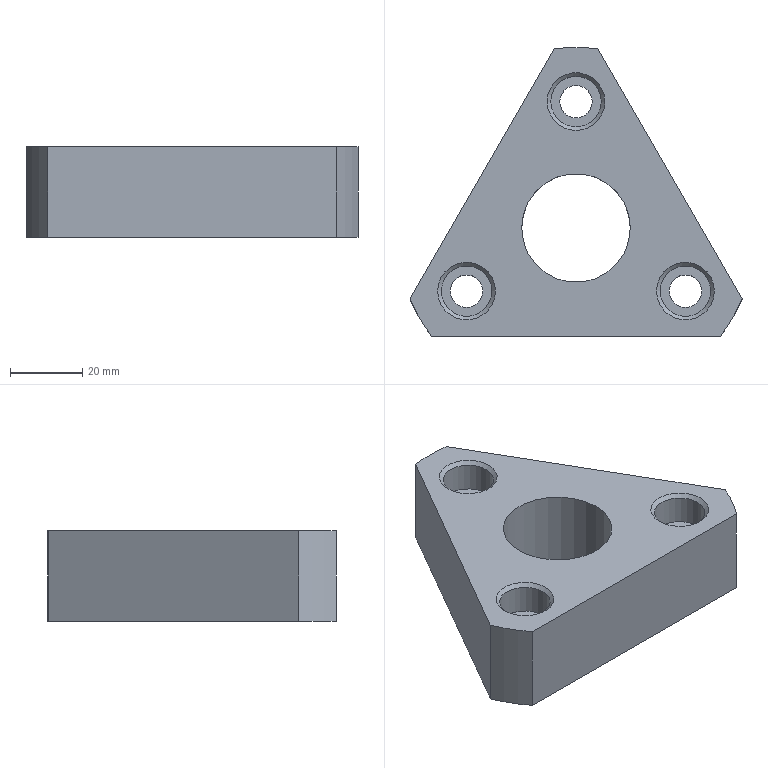NC program | NX | posted with a generic post | part box 91.962 x 80 x 25 mm
Lines 5877 to 6623 of 11626:
(ZLEVEL_PROFILE , TOOL : D10)
N11722 T10 M6
N11724 G54
N11726 G17 G0 G90 X-28.502 Y-26.671 S3000 M3
N11728 G43 Z30. H10
N11730 Z2.
N11732 G94 G1 X-28.584 Y-26.447 Z1.994 F1000.
N11734 X-29.091 Y-25.883 Z1.974
N11736 X-29.773 Y-25.55 Z1.954
N11738 X-30.128 Y-25.517 Z1.945
N11740 X-30.436 Y-25.474 Z1.937
N11742 X-30.736 Y-25.519 Z1.929
N11744 X-31.068 Y-25.672 Z1.919
N11746 X-31.388 Y-25.8 Z1.91
N11748 X-31.928 Y-26.291 Z1.891
N11750 X-32.255 Y-26.944 Z1.872
N11752 X-32.292 Y-27.286 Z1.863
N11754 X-32.325 Y-27.518 Z1.857
N11756 X-32.211 Y-28.178 Z1.839
N11758 X-31.886 Y-28.758 Z1.822
N11760 X-31.388 Y-29.199 Z1.804
N11762 X-31.068 Y-29.328 Z1.795
N11764 X-30.595 Y-29.446 Z1.782
N11766 X-30.449 Y-29.483 Z1.779
N11768 X-30.113 Y-29.481 Z1.77
N11770 X-29.771 Y-29.451 Z1.761
N11772 X-29.121 Y-29.141 Z1.742
N11774 X-28.626 Y-28.618 Z1.723
N11776 X-28.472 Y-28.252 Z1.713
N11778 X-28.337 Y-27.96 Z1.704
N11780 X-28.329 Y-27.504 Z1.692
N11782 X-28.324 Y-27.16 Z1.683
N11784 X-28.584 Y-26.447 Z1.663
N11786 X-29.091 Y-25.883 Z1.643
N11788 X-29.773 Y-25.55 Z1.624
N11790 X-30.128 Y-25.517 Z1.614
N11792 X-30.436 Y-25.474 Z1.606
N11794 X-30.736 Y-25.519 Z1.598
N11796 X-31.068 Y-25.672 Z1.589
N11798 X-31.388 Y-25.8 Z1.58
N11800 X-31.928 Y-26.291 Z1.56
N11802 X-32.255 Y-26.944 Z1.541
N11804 X-32.292 Y-27.286 Z1.532
N11806 X-32.325 Y-27.518 Z1.526
N11808 X-32.211 Y-28.178 Z1.509
N11810 X-31.886 Y-28.758 Z1.491
N11812 X-31.388 Y-29.199 Z1.474
N11814 X-31.068 Y-29.328 Z1.465
N11816 X-30.595 Y-29.446 Z1.452
N11818 X-30.449 Y-29.483 Z1.448
N11820 X-30.113 Y-29.481 Z1.439
N11822 X-29.771 Y-29.451 Z1.43
N11824 X-29.121 Y-29.141 Z1.411
N11826 X-28.626 Y-28.618 Z1.393
N11828 X-28.472 Y-28.252 Z1.382
N11830 X-28.337 Y-27.96 Z1.374
N11832 X-28.329 Y-27.504 Z1.362
N11834 X-28.324 Y-27.16 Z1.353
N11836 X-28.584 Y-26.447 Z1.333
N11838 X-29.091 Y-25.883 Z1.313
N11840 X-29.773 Y-25.55 Z1.293
N11842 X-30.128 Y-25.517 Z1.284
N11844 X-30.436 Y-25.474 Z1.276
N11846 X-30.736 Y-25.519 Z1.268
N11848 X-31.068 Y-25.672 Z1.258
N11850 X-31.388 Y-25.8 Z1.249
N11852 X-31.928 Y-26.291 Z1.23
N11854 X-32.255 Y-26.944 Z1.211
N11856 X-32.292 Y-27.286 Z1.202
N11858 X-32.325 Y-27.518 Z1.196
N11860 X-32.211 Y-28.178 Z1.178
N11862 X-31.886 Y-28.758 Z1.161
N11864 X-31.388 Y-29.199 Z1.143
N11866 X-31.068 Y-29.328 Z1.134
N11868 X-30.595 Y-29.446 Z1.122
N11870 X-30.449 Y-29.483 Z1.118
N11872 X-30.113 Y-29.481 Z1.109
N11874 X-29.771 Y-29.451 Z1.1
N11876 X-29.121 Y-29.141 Z1.081
N11878 X-28.626 Y-28.618 Z1.062
N11880 X-28.472 Y-28.252 Z1.052
N11882 X-28.337 Y-27.96 Z1.043
N11884 X-28.329 Y-27.504 Z1.031
N11886 X-28.324 Y-27.16 Z1.022
N11888 X-28.584 Y-26.447 Z1.003
N11890 X-29.091 Y-25.883 Z0.983
N11892 X-29.773 Y-25.55 Z0.963
N11894 X-30.128 Y-25.517 Z0.953
N11896 X-30.436 Y-25.474 Z0.945
N11898 X-30.736 Y-25.519 Z0.937
N11900 X-31.068 Y-25.672 Z0.928
N11902 X-31.388 Y-25.8 Z0.919
N11904 X-31.928 Y-26.291 Z0.9
N11906 X-32.255 Y-26.944 Z0.881
N11908 X-32.292 Y-27.286 Z0.872
N11910 X-32.325 Y-27.518 Z0.865
N11912 X-32.211 Y-28.178 Z0.848
N11914 X-31.886 Y-28.758 Z0.83
N11916 X-31.388 Y-29.199 Z0.813
N11918 X-31.068 Y-29.328 Z0.804
N11920 X-30.595 Y-29.446 Z0.791
N11922 X-30.449 Y-29.483 Z0.787
N11924 X-30.113 Y-29.481 Z0.778
N11926 X-29.771 Y-29.451 Z0.769
N11928 X-29.121 Y-29.141 Z0.751
N11930 X-28.626 Y-28.618 Z0.732
N11932 X-28.472 Y-28.252 Z0.721
N11934 X-28.337 Y-27.96 Z0.713
N11936 X-28.329 Y-27.504 Z0.701
N11938 X-28.324 Y-27.16 Z0.692
N11940 X-28.584 Y-26.447 Z0.672
N11942 X-29.091 Y-25.883 Z0.652
N11944 X-29.773 Y-25.55 Z0.632
N11946 X-30.128 Y-25.517 Z0.623
N11948 X-30.436 Y-25.474 Z0.615
N11950 X-30.736 Y-25.519 Z0.607
N11952 X-31.068 Y-25.672 Z0.597
N11954 X-31.388 Y-25.8 Z0.588
N11956 X-31.928 Y-26.291 Z0.569
N11958 X-32.255 Y-26.944 Z0.55
N11960 X-32.292 Y-27.286 Z0.541
N11962 X-32.325 Y-27.518 Z0.535
N11964 X-32.211 Y-28.178 Z0.517
N11966 X-31.886 Y-28.758 Z0.5
N11968 X-31.388 Y-29.199 Z0.483
N11970 X-31.068 Y-29.328 Z0.474
N11972 X-30.595 Y-29.446 Z0.461
N11974 X-30.449 Y-29.483 Z0.457
N11976 X-30.113 Y-29.481 Z0.448
N11978 X-29.771 Y-29.451 Z0.439
N11980 X-29.121 Y-29.141 Z0.42
N11982 X-28.626 Y-28.618 Z0.401
N11984 X-28.472 Y-28.252 Z0.391
N11986 X-28.337 Y-27.96 Z0.383
N11988 X-28.329 Y-27.504 Z0.371
N11990 X-28.324 Y-27.16 Z0.362
N11992 X-28.584 Y-26.447 Z0.342
N11994 X-29.091 Y-25.883 Z0.322
N11996 X-29.773 Y-25.55 Z0.302
N11998 X-30.128 Y-25.517 Z0.293
N12000 X-30.436 Y-25.474 Z0.284
N12002 X-30.736 Y-25.519 Z0.277
N12004 X-31.068 Y-25.672 Z0.267
N12006 X-31.388 Y-25.8 Z0.258
N12008 X-31.928 Y-26.291 Z0.239
N12010 X-32.255 Y-26.944 Z0.22
N12012 X-32.292 Y-27.286 Z0.211
N12014 X-32.325 Y-27.518 Z0.205
N12016 X-32.211 Y-28.178 Z0.187
N12018 X-31.886 Y-28.758 Z0.17
N12020 X-31.388 Y-29.199 Z0.152
N12022 X-31.068 Y-29.328 Z0.143
N12024 X-30.595 Y-29.446 Z0.13
N12026 X-30.449 Y-29.483 Z0.126
N12028 X-30.113 Y-29.481 Z0.118
N12030 X-29.771 Y-29.451 Z0.109
N12032 X-29.121 Y-29.141 Z0.09
N12034 X-28.626 Y-28.618 Z0.071
N12036 X-28.472 Y-28.252 Z0.061
N12038 X-28.337 Y-27.96 Z0.052
N12040 X-28.329 Y-27.504 Z0.04
N12042 X-28.324 Y-27.16 Z0.031
N12044 X-28.584 Y-26.447 Z0.011
N12046 X-29.091 Y-25.883 Z-0.009
N12048 X-29.773 Y-25.55 Z-0.028
N12050 X-30.128 Y-25.517 Z-0.038
N12052 X-30.436 Y-25.474 Z-0.046
N12054 X-30.736 Y-25.519 Z-0.054
N12056 X-31.068 Y-25.672 Z-0.063
N12058 X-31.388 Y-25.8 Z-0.072
N12060 X-31.928 Y-26.291 Z-0.092
N12062 X-32.255 Y-26.944 Z-0.111
N12064 X-32.292 Y-27.286 Z-0.12
N12066 X-32.325 Y-27.518 Z-0.126
N12068 X-32.211 Y-28.178 Z-0.143
N12070 X-31.886 Y-28.758 Z-0.161
N12072 X-31.388 Y-29.199 Z-0.178
N12074 X-31.068 Y-29.328 Z-0.187
N12076 X-30.595 Y-29.446 Z-0.2
N12078 X-30.449 Y-29.483 F1800.
N12080 X-30.113 Y-29.481
N12082 G3 X-28.472 Y-28.252 R1.942
N12084 G1 X-28.337 Y-27.96
N12086 X-28.329 Y-27.504
N12088 G3 X-30.128 Y-25.517 R1.965
N12090 X-31.068 Y-25.672 R1.599
N12092 X-32.292 Y-27.286 R1.965
N12094 G1 X-32.325 Y-27.518
N12096 X-32.27 Y-27.838
N12098 G3 X-31.068 Y-29.328 R1.967
N12100 G1 X-30.595 Y-29.446
N12102 X-30.224 Y-29.485 Z-0.208
N12104 X-29.853 Y-29.441 Z-0.216
N12106 X-29.497 Y-29.323 Z-0.224
N12108 X-29.17 Y-29.139 Z-0.232
N12110 X-28.885 Y-28.896 Z-0.24
N12112 X-28.652 Y-28.602 Z-0.248
N12114 X-28.48 Y-28.269 Z-0.256
N12116 X-28.336 Y-27.925 Z-0.264
N12118 X-28.33 Y-27.55 Z-0.272
N12120 X-28.352 Y-27.176 Z-0.28
N12122 X-28.444 Y-26.812 Z-0.288
N12124 X-28.603 Y-26.473 Z-0.296
N12126 X-28.825 Y-26.17 Z-0.304
N12128 X-29.099 Y-25.915 Z-0.312
N12130 X-29.417 Y-25.717 Z-0.32
N12132 X-29.767 Y-25.583 Z-0.328
N12134 X-30.136 Y-25.516 Z-0.336
N12136 X-30.511 Y-25.51 Z-0.344
N12138 X-30.876 Y-25.592 Z-0.352
N12140 X-31.221 Y-25.741 Z-0.36
N12142 X-31.538 Y-25.941 Z-0.368
N12144 X-31.812 Y-26.197 Z-0.376
N12146 X-32.032 Y-26.5 Z-0.384
N12148 X-32.19 Y-26.84 Z-0.392
N12150 X-32.281 Y-27.204 Z-0.4
N12152 X-32.325 Y-27.518
N12154 X-32.27 Y-27.838
N12156 G3 X-31.068 Y-29.328 R1.967
N12158 G1 X-30.595 Y-29.446
N12160 X-30.224 Y-29.485 Z-0.408
N12162 X-29.853 Y-29.441 Z-0.416
N12164 X-29.497 Y-29.323 Z-0.424
N12166 X-29.17 Y-29.139 Z-0.432
N12168 X-28.885 Y-28.896 Z-0.44
N12170 X-28.652 Y-28.602 Z-0.448
N12172 X-28.48 Y-28.269 Z-0.456
N12174 X-28.336 Y-27.925 Z-0.464
N12176 X-28.33 Y-27.55 Z-0.472
N12178 X-28.352 Y-27.176 Z-0.48
N12180 X-28.444 Y-26.812 Z-0.488
N12182 X-28.603 Y-26.473 Z-0.496
N12184 X-28.825 Y-26.17 Z-0.504
N12186 X-29.099 Y-25.915 Z-0.512
N12188 X-29.417 Y-25.717 Z-0.52
N12190 X-29.767 Y-25.583 Z-0.528
N12192 X-30.136 Y-25.516 Z-0.536
N12194 X-30.511 Y-25.51 Z-0.544
N12196 X-30.876 Y-25.592 Z-0.552
N12198 X-31.221 Y-25.741 Z-0.56
N12200 X-31.538 Y-25.941 Z-0.568
N12202 X-31.812 Y-26.197 Z-0.576
N12204 X-32.032 Y-26.5 Z-0.584
N12206 X-32.19 Y-26.84 Z-0.592
N12208 X-32.281 Y-27.204 Z-0.6
N12210 X-32.325 Y-27.518
N12212 X-32.27 Y-27.838
N12214 G3 X-31.068 Y-29.328 R1.967
N12216 G1 X-30.595 Y-29.446
N12218 X-30.224 Y-29.485 Z-0.608
N12220 X-29.853 Y-29.441 Z-0.616
N12222 X-29.497 Y-29.323 Z-0.624
N12224 X-29.17 Y-29.139 Z-0.632
N12226 X-28.885 Y-28.896 Z-0.64
N12228 X-28.652 Y-28.602 Z-0.648
N12230 X-28.48 Y-28.269 Z-0.656
N12232 X-28.336 Y-27.925 Z-0.664
N12234 X-28.33 Y-27.55 Z-0.672
N12236 X-28.352 Y-27.176 Z-0.68
N12238 X-28.444 Y-26.812 Z-0.688
N12240 X-28.603 Y-26.473 Z-0.696
N12242 X-28.825 Y-26.17 Z-0.704
N12244 X-29.099 Y-25.915 Z-0.712
N12246 X-29.417 Y-25.717 Z-0.72
N12248 X-29.767 Y-25.583 Z-0.728
N12250 X-30.136 Y-25.516 Z-0.736
N12252 X-30.511 Y-25.51 Z-0.744
N12254 X-30.876 Y-25.592 Z-0.752
N12256 X-31.221 Y-25.741 Z-0.76
N12258 X-31.538 Y-25.941 Z-0.768
N12260 X-31.812 Y-26.197 Z-0.776
N12262 X-32.032 Y-26.5 Z-0.784
N12264 X-32.19 Y-26.84 Z-0.792
N12266 X-32.281 Y-27.204 Z-0.8
N12268 X-32.325 Y-27.519
N12270 X-32.27 Y-27.838
N12272 G3 X-31.068 Y-29.328 R1.967
N12274 G1 X-30.595 Y-29.446
N12276 X-30.224 Y-29.485 Z-0.808
N12278 X-29.853 Y-29.441 Z-0.816
N12280 X-29.497 Y-29.323 Z-0.824
N12282 X-29.17 Y-29.139 Z-0.832
N12284 X-28.885 Y-28.896 Z-0.84
N12286 X-28.652 Y-28.602 Z-0.848
N12288 X-28.48 Y-28.269 Z-0.856
N12290 X-28.336 Y-27.925 Z-0.864
N12292 X-28.33 Y-27.55 Z-0.872
N12294 X-28.352 Y-27.176 Z-0.88
N12296 X-28.444 Y-26.812 Z-0.888
N12298 X-28.603 Y-26.473 Z-0.896
N12300 X-28.825 Y-26.17 Z-0.904
N12302 X-29.099 Y-25.915 Z-0.912
N12304 X-29.417 Y-25.717 Z-0.92
N12306 X-29.767 Y-25.583 Z-0.928
N12308 X-30.136 Y-25.516 Z-0.936
N12310 X-30.511 Y-25.51 Z-0.944
N12312 X-30.876 Y-25.592 Z-0.952
N12314 X-31.221 Y-25.741 Z-0.96
N12316 X-31.538 Y-25.941 Z-0.968
N12318 X-31.812 Y-26.197 Z-0.976
N12320 X-32.032 Y-26.5 Z-0.984
N12322 X-32.19 Y-26.84 Z-0.992
N12324 X-32.281 Y-27.204 Z-1.
N12326 X-32.325 Y-27.519
N12328 X-32.27 Y-27.838
N12330 G3 X-31.068 Y-29.328 R1.966
N12332 G1 X-30.595 Y-29.446
N12334 X-30.305 Y-29.486 Z-1.006
N12336 X-30.16 Y-29.494 Z-1.009
N12338 X-29.881 Y-29.445 Z-1.015
N12340 X-29.579 Y-29.361 Z-1.022
N12342 X-29.438 Y-29.299 Z-1.025
N12344 X-29.362 Y-29.261 Z-1.027
N12346 X-29.216 Y-29.174 Z-1.031
N12348 X-28.987 Y-28.999 Z-1.037
N12350 X-28.818 Y-28.831 Z-1.042
N12352 X-28.705 Y-28.671 Z-1.046
N12354 X-28.539 Y-28.393 Z-1.053
N12356 X-28.471 Y-28.248 Z-1.056
N12358 X-28.443 Y-28.174 Z-1.058
N12360 X-28.4 Y-28.02 Z-1.062
N12362 X-28.348 Y-27.724 Z-1.068
N12364 X-28.329 Y-27.49 Z-1.073
N12366 X-28.343 Y-27.32 Z-1.077
N12368 X-28.395 Y-27.002 Z-1.084
N12370 X-28.436 Y-26.849 Z-1.087
N12372 X-28.461 Y-26.773 Z-1.089
N12374 X-28.529 Y-26.629 Z-1.092
N12376 X-28.686 Y-26.355 Z-1.099
N12378 X-28.772 Y-26.223 Z-1.102
N12380 X-28.825 Y-26.161 Z-1.104
N12382 X-28.948 Y-26.049 Z-1.108
N12384 X-29.213 Y-25.828 Z-1.115
N12386 X-29.42 Y-25.71 Z-1.12
N12388 X-29.547 Y-25.652 Z-1.123
N12390 X-29.967 Y-25.542 Z-1.132
N12392 X-30.252 Y-25.513 Z-1.138
N12394 X-30.526 Y-25.523 Z-1.144
N12396 X-30.759 Y-25.57 Z-1.149
N12398 X-30.955 Y-25.629 Z-1.154
N12400 X-31.352 Y-25.822 Z-1.163
N12402 X-31.58 Y-25.981 Z-1.169
N12404 X-31.786 Y-26.169 Z-1.175
N12406 X-31.934 Y-26.356 Z-1.18
N12408 X-32.043 Y-26.527 Z-1.185
N12410 X-32.192 Y-26.856 Z-1.192
N12412 X-32.289 Y-27.203 Z-1.2
N12414 G3 X-30.6 Y-29.479 R2.
N12416 G1 X-30.138 Y-29.493 Z-1.21
N12418 X-29.881 Y-29.445 Z-1.215
N12420 X-29.575 Y-29.36 Z-1.222
N12422 X-29.432 Y-29.296 Z-1.225
N12424 X-29.358 Y-29.258 Z-1.227
N12426 X-29.215 Y-29.173 Z-1.231
N12428 X-28.985 Y-28.997 Z-1.237
N12430 X-28.815 Y-28.828 Z-1.242
N12432 X-28.703 Y-28.668 Z-1.246
N12434 X-28.538 Y-28.393 Z-1.253
N12436 X-28.471 Y-28.249 Z-1.256
N12438 X-28.443 Y-28.174 Z-1.258
N12440 X-28.4 Y-28.02 Z-1.262
N12442 X-28.347 Y-27.719 Z-1.268
N12444 X-28.33 Y-27.481 Z-1.273
N12446 X-28.344 Y-27.309 Z-1.277
N12448 X-28.397 Y-26.996 Z-1.284
N12450 X-28.437 Y-26.844 Z-1.287
N12452 X-28.463 Y-26.767 Z-1.289
N12454 X-28.533 Y-26.621 Z-1.292
N12456 X-28.694 Y-26.344 Z-1.299
N12458 X-28.781 Y-26.211 Z-1.302
N12460 X-28.835 Y-26.151 Z-1.304
N12462 X-28.955 Y-26.042 Z-1.308
N12464 X-29.225 Y-25.821 Z-1.315
N12466 X-29.433 Y-25.703 Z-1.32
N12468 X-29.557 Y-25.648 Z-1.323
N12470 X-29.98 Y-25.539 Z-1.332
N12472 X-30.263 Y-25.513 Z-1.338
N12474 X-30.537 Y-25.526 Z-1.344
N12476 X-30.77 Y-25.573 Z-1.349
N12478 X-30.968 Y-25.633 Z-1.354
N12480 X-31.362 Y-25.826 Z-1.363
N12482 X-31.587 Y-25.988 Z-1.369
N12484 X-31.794 Y-26.179 Z-1.375
N12486 X-31.942 Y-26.366 Z-1.38
N12488 X-32.047 Y-26.535 Z-1.385
N12490 X-32.195 Y-26.864 Z-1.392
N12492 X-32.29 Y-27.211 Z-1.4
N12494 G3 X-30.6 Y-29.479 R2.
N12496 G1 X-30.139 Y-29.484 Z-1.41
N12498 X-29.881 Y-29.445 Z-1.415
N12500 X-29.59 Y-29.365 Z-1.422
N12502 X-29.453 Y-29.307 Z-1.425
N12504 X-29.372 Y-29.266 Z-1.427
N12506 X-29.215 Y-29.173 Z-1.431
N12508 X-28.986 Y-28.999 Z-1.437
N12510 X-28.817 Y-28.829 Z-1.442
N12512 X-28.703 Y-28.668 Z-1.446
N12514 X-28.538 Y-28.393 Z-1.453
N12516 X-28.471 Y-28.25 Z-1.456
N12518 X-28.444 Y-28.175 Z-1.458
N12520 X-28.4 Y-28.02 Z-1.462
N12522 X-28.347 Y-27.719 Z-1.468
N12524 X-28.33 Y-27.482 Z-1.473
N12526 X-28.344 Y-27.309 Z-1.477
N12528 X-28.397 Y-26.996 Z-1.484
N12530 X-28.437 Y-26.844 Z-1.487
N12532 X-28.463 Y-26.767 Z-1.489
N12534 X-28.533 Y-26.621 Z-1.492
N12536 X-28.694 Y-26.345 Z-1.499
N12538 X-28.781 Y-26.212 Z-1.502
N12540 X-28.834 Y-26.151 Z-1.504
N12542 X-28.955 Y-26.042 Z-1.508
N12544 X-29.225 Y-25.821 Z-1.515
N12546 X-29.433 Y-25.703 Z-1.52
N12548 X-29.557 Y-25.648 Z-1.523
N12550 X-29.98 Y-25.54 Z-1.532
N12552 X-30.263 Y-25.513 Z-1.538
N12554 X-30.537 Y-25.524 Z-1.544
N12556 X-30.771 Y-25.571 Z-1.549
N12558 X-30.968 Y-25.634 Z-1.554
N12560 X-31.366 Y-25.83 Z-1.563
N12562 X-31.587 Y-25.988 Z-1.569
N12564 X-31.793 Y-26.178 Z-1.575
N12566 X-31.941 Y-26.365 Z-1.58
N12568 X-32.047 Y-26.535 Z-1.585
N12570 X-32.195 Y-26.864 Z-1.592
N12572 X-32.29 Y-27.211 Z-1.6
N12574 G3 X-30.6 Y-29.479 R2.
N12576 G1 X-30.139 Y-29.484 Z-1.61
N12578 X-29.881 Y-29.445 Z-1.615
N12580 X-29.59 Y-29.365 Z-1.622
N12582 X-29.453 Y-29.307 Z-1.625
N12584 X-29.372 Y-29.266 Z-1.627
N12586 X-29.215 Y-29.173 Z-1.631
N12588 X-28.986 Y-28.999 Z-1.637
N12590 X-28.817 Y-28.829 Z-1.642
N12592 X-28.703 Y-28.668 Z-1.646
N12594 X-28.538 Y-28.393 Z-1.653
N12596 X-28.471 Y-28.249 Z-1.656
N12598 X-28.444 Y-28.175 Z-1.658
N12600 X-28.4 Y-28.02 Z-1.662
N12602 X-28.347 Y-27.719 Z-1.668
N12604 X-28.33 Y-27.482 Z-1.673
N12606 X-28.344 Y-27.309 Z-1.677
N12608 X-28.397 Y-26.996 Z-1.684
N12610 X-28.437 Y-26.844 Z-1.687
N12612 X-28.463 Y-26.768 Z-1.689
N12614 X-28.533 Y-26.621 Z-1.692
N12616 X-28.694 Y-26.345 Z-1.699
N12618 X-28.781 Y-26.212 Z-1.702
N12620 X-28.834 Y-26.151 Z-1.704
N12622 X-28.955 Y-26.042 Z-1.708
N12624 X-29.225 Y-25.821 Z-1.715
N12626 X-29.433 Y-25.703 Z-1.72
N12628 X-29.557 Y-25.648 Z-1.723
N12630 X-29.98 Y-25.54 Z-1.732
N12632 X-30.263 Y-25.513 Z-1.738
N12634 X-30.537 Y-25.524 Z-1.744
N12636 X-30.771 Y-25.571 Z-1.749
N12638 X-30.968 Y-25.634 Z-1.754
N12640 X-31.366 Y-25.83 Z-1.763
N12642 X-31.587 Y-25.988 Z-1.769
N12644 X-31.793 Y-26.178 Z-1.775
N12646 X-31.94 Y-26.365 Z-1.78
N12648 X-32.047 Y-26.535 Z-1.785
N12650 X-32.195 Y-26.864 Z-1.792
N12652 X-32.29 Y-27.211 Z-1.8
N12654 G3 X-30.6 Y-29.479 R2.
N12656 G1 X-30.14 Y-29.484 Z-1.81
N12658 X-29.881 Y-29.445 Z-1.815
N12660 X-29.59 Y-29.365 Z-1.822
N12662 X-29.453 Y-29.307 Z-1.825
N12664 X-29.372 Y-29.266 Z-1.827
N12666 X-29.215 Y-29.173 Z-1.831
N12668 X-28.986 Y-28.999 Z-1.837
N12670 X-28.817 Y-28.829 Z-1.842
N12672 X-28.703 Y-28.668 Z-1.846
N12674 X-28.538 Y-28.393 Z-1.853
N12676 X-28.471 Y-28.249 Z-1.856
N12678 X-28.444 Y-28.174 Z-1.858
N12680 X-28.4 Y-28.02 Z-1.862
N12682 X-28.347 Y-27.719 Z-1.868
N12684 X-28.33 Y-27.482 Z-1.873
N12686 X-28.345 Y-27.309 Z-1.877
N12688 X-28.397 Y-26.996 Z-1.884
N12690 X-28.437 Y-26.845 Z-1.887
N12692 X-28.463 Y-26.768 Z-1.889
N12694 X-28.533 Y-26.621 Z-1.892
N12696 X-28.694 Y-26.345 Z-1.899
N12698 X-28.781 Y-26.212 Z-1.902
N12700 X-28.834 Y-26.151 Z-1.904
N12702 X-28.955 Y-26.042 Z-1.908
N12704 X-29.225 Y-25.82 Z-1.915
N12706 X-29.433 Y-25.703 Z-1.92
N12708 X-29.557 Y-25.648 Z-1.923
N12710 X-29.98 Y-25.54 Z-1.932
N12712 X-30.263 Y-25.513 Z-1.938
N12714 X-30.537 Y-25.524 Z-1.944
N12716 X-30.771 Y-25.571 Z-1.949
N12718 X-30.968 Y-25.634 Z-1.954
N12720 X-31.366 Y-25.83 Z-1.963
N12722 X-31.587 Y-25.988 Z-1.969
N12724 X-31.793 Y-26.178 Z-1.975
N12726 X-31.94 Y-26.365 Z-1.98
N12728 X-32.047 Y-26.535 Z-1.985
N12730 X-32.195 Y-26.864 Z-1.992
N12732 X-32.29 Y-27.211 Z-2.
N12734 G3 X-30.6 Y-29.479 R2.
N12736 G1 X-30.14 Y-29.484 Z-2.01
N12738 X-29.881 Y-29.445 Z-2.015
N12740 X-29.59 Y-29.365 Z-2.022
N12742 X-29.453 Y-29.307 Z-2.025
N12744 X-29.372 Y-29.266 Z-2.027
N12746 X-29.215 Y-29.173 Z-2.031
N12748 X-28.986 Y-28.999 Z-2.037
N12750 X-28.817 Y-28.829 Z-2.042
N12752 X-28.703 Y-28.668 Z-2.046
N12754 X-28.538 Y-28.393 Z-2.053
N12756 X-28.471 Y-28.249 Z-2.056
N12758 X-28.444 Y-28.174 Z-2.058
N12760 X-28.4 Y-28.02 Z-2.062
N12762 X-28.347 Y-27.719 Z-2.068
N12764 X-28.33 Y-27.482 Z-2.073
N12766 X-28.345 Y-27.309 Z-2.077
N12768 X-28.397 Y-26.996 Z-2.084
N12770 X-28.437 Y-26.845 Z-2.087
N12772 X-28.463 Y-26.768 Z-2.089
N12774 X-28.533 Y-26.621 Z-2.092
N12776 X-28.694 Y-26.346 Z-2.099
N12778 X-28.78 Y-26.213 Z-2.102
N12780 X-28.834 Y-26.152 Z-2.104
N12782 X-28.955 Y-26.042 Z-2.108
N12784 X-29.225 Y-25.82 Z-2.115
N12786 X-29.433 Y-25.703 Z-2.12
N12788 X-29.557 Y-25.648 Z-2.123
N12790 X-29.98 Y-25.54 Z-2.132
N12792 X-30.263 Y-25.513 Z-2.138
N12794 X-30.537 Y-25.524 Z-2.144
N12796 X-30.77 Y-25.571 Z-2.149
N12798 X-30.968 Y-25.634 Z-2.154
N12800 X-31.366 Y-25.829 Z-2.163
N12802 X-31.587 Y-25.988 Z-2.169
N12804 X-31.795 Y-26.179 Z-2.175
N12806 X-31.942 Y-26.367 Z-2.18
N12808 X-32.047 Y-26.535 Z-2.185
N12810 X-32.195 Y-26.864 Z-2.192
N12812 X-32.29 Y-27.211 Z-2.2
N12814 G3 X-30.6 Y-29.479 R2.
N12816 G1 X-30.14 Y-29.484 Z-2.21
N12818 X-29.881 Y-29.445 Z-2.215
N12820 X-29.59 Y-29.365 Z-2.222
N12822 X-29.453 Y-29.307 Z-2.225
N12824 X-29.372 Y-29.266 Z-2.227
N12826 X-29.215 Y-29.173 Z-2.231
N12828 X-28.986 Y-28.999 Z-2.237
N12830 X-28.817 Y-28.829 Z-2.242
N12832 X-28.703 Y-28.668 Z-2.246
N12834 X-28.538 Y-28.393 Z-2.253
N12836 X-28.471 Y-28.249 Z-2.256
N12838 X-28.444 Y-28.174 Z-2.258
N12840 X-28.4 Y-28.02 Z-2.262
N12842 X-28.347 Y-27.719 Z-2.268
N12844 X-28.33 Y-27.482 Z-2.273
N12846 X-28.345 Y-27.309 Z-2.277
N12848 X-28.397 Y-26.997 Z-2.284
N12850 X-28.437 Y-26.845 Z-2.287
N12852 X-28.463 Y-26.768 Z-2.289
N12854 X-28.533 Y-26.621 Z-2.292
N12856 X-28.694 Y-26.346 Z-2.299
N12858 X-28.78 Y-26.213 Z-2.302
N12860 X-28.834 Y-26.152 Z-2.304
N12862 X-28.955 Y-26.042 Z-2.308
N12864 X-29.225 Y-25.82 Z-2.315
N12866 X-29.433 Y-25.703 Z-2.32
N12868 X-29.557 Y-25.648 Z-2.323
N12870 X-29.98 Y-25.54 Z-2.332
N12872 X-30.263 Y-25.513 Z-2.338
N12874 X-30.537 Y-25.524 Z-2.344
N12876 X-30.77 Y-25.572 Z-2.349
N12878 X-30.968 Y-25.634 Z-2.354
N12880 X-31.366 Y-25.829 Z-2.363
N12882 X-31.587 Y-25.988 Z-2.369
N12884 X-31.794 Y-26.179 Z-2.375
N12886 X-31.942 Y-26.367 Z-2.38
N12888 X-32.047 Y-26.535 Z-2.385
N12890 X-32.195 Y-26.864 Z-2.392
N12892 X-32.29 Y-27.211 Z-2.4
N12894 G3 X-30.6 Y-29.479 R2.
N12896 G1 X-30.14 Y-29.484 Z-2.41
N12898 X-29.881 Y-29.445 Z-2.415
N12900 X-29.59 Y-29.365 Z-2.422
N12902 X-29.453 Y-29.307 Z-2.425
N12904 X-29.372 Y-29.266 Z-2.427
N12906 X-29.215 Y-29.173 Z-2.431
N12908 X-28.986 Y-28.999 Z-2.437
N12910 X-28.817 Y-28.829 Z-2.442
N12912 X-28.703 Y-28.668 Z-2.446
N12914 X-28.538 Y-28.393 Z-2.453
N12916 X-28.471 Y-28.249 Z-2.456
N12918 X-28.444 Y-28.174 Z-2.458
N12920 X-28.4 Y-28.02 Z-2.462
N12922 X-28.347 Y-27.719 Z-2.468
N12924 X-28.331 Y-27.482 Z-2.473
N12926 X-28.345 Y-27.309 Z-2.477
N12928 X-28.397 Y-26.997 Z-2.484
N12930 X-28.437 Y-26.845 Z-2.487
N12932 X-28.463 Y-26.768 Z-2.489
N12934 X-28.533 Y-26.621 Z-2.492
N12936 X-28.694 Y-26.346 Z-2.499
N12938 X-28.78 Y-26.213 Z-2.502
N12940 X-28.834 Y-26.152 Z-2.504
N12942 X-28.955 Y-26.042 Z-2.508
N12944 X-29.225 Y-25.82 Z-2.515
N12946 X-29.433 Y-25.703 Z-2.52
N12948 X-29.557 Y-25.648 Z-2.523
N12950 X-29.98 Y-25.54 Z-2.532
N12952 X-30.263 Y-25.513 Z-2.538
N12954 X-30.537 Y-25.524 Z-2.544
N12956 X-30.77 Y-25.572 Z-2.549
N12958 X-30.968 Y-25.634 Z-2.554
N12960 X-31.366 Y-25.829 Z-2.563
N12962 X-31.587 Y-25.988 Z-2.569
N12964 X-31.794 Y-26.179 Z-2.575
N12966 X-31.942 Y-26.367 Z-2.58
N12968 X-32.047 Y-26.535 Z-2.585
N12970 X-32.195 Y-26.864 Z-2.592
N12972 X-32.29 Y-27.211 Z-2.6
N12974 G3 X-30.6 Y-29.479 R2.
N12976 G1 X-30.14 Y-29.484 Z-2.61
N12978 X-29.881 Y-29.445 Z-2.615
N12980 X-29.59 Y-29.365 Z-2.622
N12982 X-29.453 Y-29.307 Z-2.625
N12984 X-29.372 Y-29.266 Z-2.627
N12986 X-29.215 Y-29.173 Z-2.631
N12988 X-28.987 Y-28.999 Z-2.637
N12990 X-28.817 Y-28.829 Z-2.642
N12992 X-28.703 Y-28.668 Z-2.646
N12994 X-28.538 Y-28.392 Z-2.653
N12996 X-28.471 Y-28.249 Z-2.656
N12998 X-28.444 Y-28.174 Z-2.658
N13000 X-28.4 Y-28.02 Z-2.662
N13002 X-28.347 Y-27.719 Z-2.668
N13004 X-28.331 Y-27.482 Z-2.673
N13006 X-28.345 Y-27.309 Z-2.677
N13008 X-28.397 Y-26.997 Z-2.684
N13010 X-28.437 Y-26.845 Z-2.687
N13012 X-28.463 Y-26.768 Z-2.689
N13014 X-28.533 Y-26.621 Z-2.692
N13016 X-28.694 Y-26.346 Z-2.699
N13018 X-28.78 Y-26.213 Z-2.702
N13020 X-28.833 Y-26.152 Z-2.704
N13022 X-28.955 Y-26.042 Z-2.708
N13024 X-29.225 Y-25.82 Z-2.715
N13026 X-29.433 Y-25.703 Z-2.72
N13028 X-29.557 Y-25.648 Z-2.723
N13030 X-29.98 Y-25.54 Z-2.732
N13032 X-30.263 Y-25.513 Z-2.738
N13034 X-30.537 Y-25.524 Z-2.744
N13036 X-30.77 Y-25.572 Z-2.749
N13038 X-30.968 Y-25.634 Z-2.754
N13040 X-31.366 Y-25.829 Z-2.763
N13042 X-31.587 Y-25.988 Z-2.769
N13044 X-31.794 Y-26.179 Z-2.775
N13046 X-31.941 Y-26.367 Z-2.78
N13048 X-32.047 Y-26.535 Z-2.785
N13050 X-32.195 Y-26.864 Z-2.792
N13052 X-32.29 Y-27.211 Z-2.8
N13054 G3 X-30.6 Y-29.479 R2.
N13056 G1 X-30.14 Y-29.484 Z-2.81
N13058 X-29.881 Y-29.445 Z-2.815
N13060 X-29.59 Y-29.365 Z-2.822
N13062 X-29.453 Y-29.307 Z-2.825
N13064 X-29.372 Y-29.266 Z-2.827
N13066 X-29.215 Y-29.173 Z-2.831
N13068 X-28.987 Y-28.999 Z-2.837
N13070 X-28.817 Y-28.829 Z-2.842
N13072 X-28.703 Y-28.668 Z-2.846
N13074 X-28.538 Y-28.392 Z-2.853
N13076 X-28.471 Y-28.248 Z-2.856
N13078 X-28.444 Y-28.174 Z-2.858
N13080 X-28.4 Y-28.02 Z-2.862
N13082 X-28.347 Y-27.719 Z-2.868
N13084 X-28.331 Y-27.482 Z-2.873
N13086 X-28.345 Y-27.309 Z-2.877
N13088 X-28.397 Y-26.997 Z-2.884
N13090 X-28.437 Y-26.845 Z-2.887
N13092 X-28.463 Y-26.768 Z-2.889
N13094 X-28.533 Y-26.621 Z-2.892
N13096 X-28.694 Y-26.346 Z-2.899
N13098 X-28.78 Y-26.213 Z-2.902
N13100 X-28.833 Y-26.152 Z-2.904
N13102 X-28.955 Y-26.042 Z-2.908
N13104 X-29.226 Y-25.82 Z-2.915
N13106 X-29.433 Y-25.703 Z-2.92
N13108 X-29.557 Y-25.648 Z-2.923
N13110 X-29.98 Y-25.54 Z-2.932
N13112 X-30.263 Y-25.513 Z-2.938
N13114 X-30.537 Y-25.524 Z-2.944
N13116 X-30.77 Y-25.572 Z-2.949
N13118 X-30.968 Y-25.634 Z-2.954
N13120 X-31.365 Y-25.829 Z-2.963
N13122 X-31.587 Y-25.988 Z-2.969
N13124 X-31.794 Y-26.179 Z-2.975
N13126 X-31.941 Y-26.366 Z-2.98
N13128 X-32.047 Y-26.535 Z-2.985
N13130 X-32.195 Y-26.864 Z-2.992
N13132 X-32.29 Y-27.211 Z-3.
N13134 G3 X-30.6 Y-29.479 R2.
N13136 G1 X-30.14 Y-29.484 Z-3.01
N13138 X-29.881 Y-29.445 Z-3.015
N13140 X-29.59 Y-29.365 Z-3.022
N13142 X-29.453 Y-29.307 Z-3.025
N13144 X-29.372 Y-29.266 Z-3.027
N13146 X-29.215 Y-29.173 Z-3.031
N13148 X-28.987 Y-28.999 Z-3.037
N13150 X-28.817 Y-28.829 Z-3.042
N13152 X-28.703 Y-28.668 Z-3.046
N13154 X-28.539 Y-28.392 Z-3.053
N13156 X-28.471 Y-28.248 Z-3.056
N13158 X-28.444 Y-28.174 Z-3.058
N13160 X-28.4 Y-28.02 Z-3.062
N13162 X-28.347 Y-27.719 Z-3.068
N13164 X-28.331 Y-27.482 Z-3.073
N13166 X-28.345 Y-27.309 Z-3.077
N13168 X-28.397 Y-26.997 Z-3.084
N13170 X-28.437 Y-26.846 Z-3.087
N13172 X-28.463 Y-26.769 Z-3.089
N13174 X-28.533 Y-26.621 Z-3.092
N13176 X-28.694 Y-26.347 Z-3.099
N13178 X-28.779 Y-26.214 Z-3.102
N13180 X-28.833 Y-26.152 Z-3.104
N13182 X-28.955 Y-26.042 Z-3.108
N13184 X-29.226 Y-25.82 Z-3.115
N13186 X-29.434 Y-25.703 Z-3.12
N13188 X-29.557 Y-25.648 Z-3.123
N13190 X-29.98 Y-25.54 Z-3.132
N13192 X-30.263 Y-25.513 Z-3.138
N13194 X-30.537 Y-25.524 Z-3.144
N13196 X-30.77 Y-25.572 Z-3.149
N13198 X-30.968 Y-25.634 Z-3.154
N13200 X-31.365 Y-25.829 Z-3.163
N13202 X-31.587 Y-25.988 Z-3.169
N13204 X-31.794 Y-26.179 Z-3.175
N13206 X-31.941 Y-26.366 Z-3.18
N13208 X-32.047 Y-26.535 Z-3.185